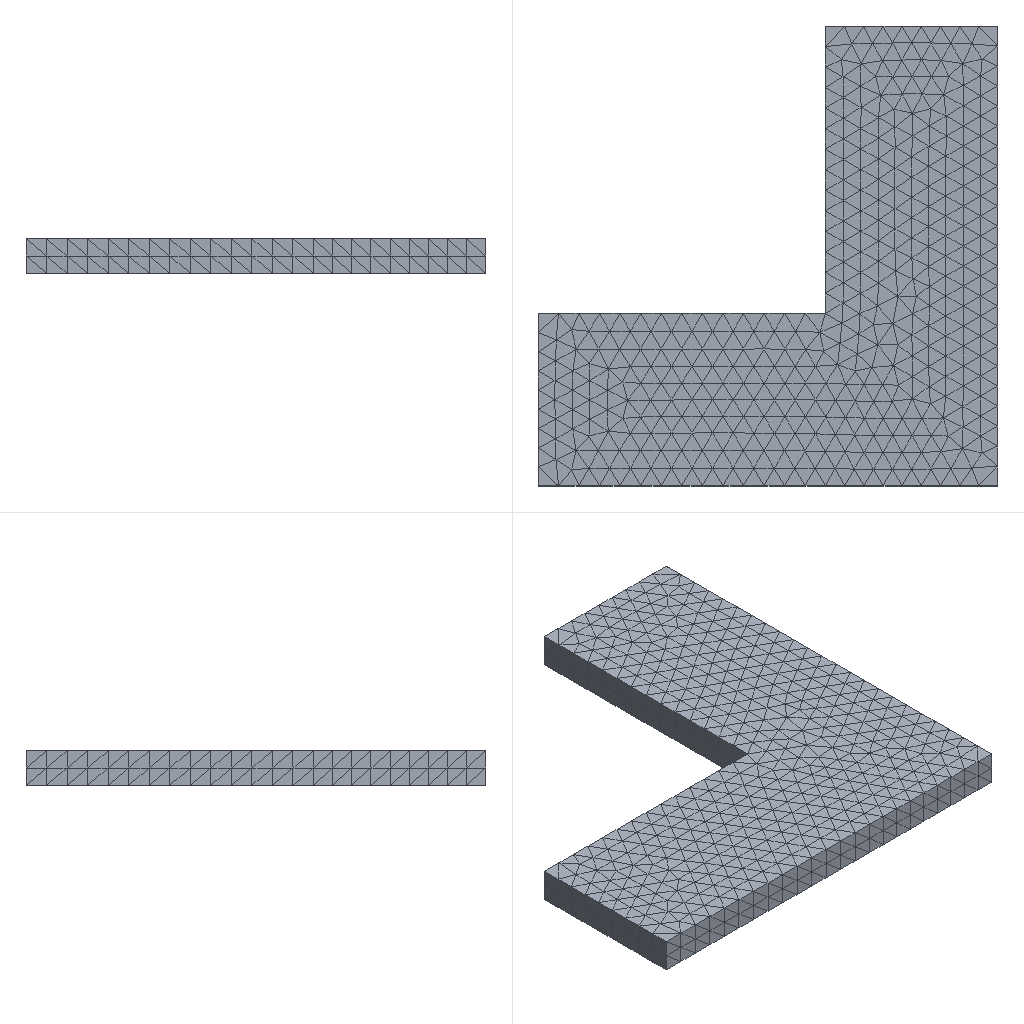Simulation study | abaqus
Notes in the study folder:
05 L bracket
job_status=None
Umax_mm=0.000139926
S_Mises_max_MPa=0.479355
Set-up summary:
category,name,step,type,value,unit,region
solver,abaqus,,Abaqus/CAE 2024
units,mm-N-s-tonne (MPa),,inferred,E=210000 density=7.85e-09
analysis,Step-1,,static,time_period=1
mesh,nodes,,,8082
mesh,elements,,,4612
element_type,C3D10,,,4612
material,Steel,,E,210000
material,Steel,,nu,0.3
material,Steel,,density,7.85e-09
section,Steel,,solid section,,,_PickedSet2
load,Load,Step-1,pressure,0.3,,LOAD
bc,BC,Step-1,encastre,[dofs=ENCASTRE],,FIXED
Abaqus input file, long lists of numbers shortened:
*Heading
** Job name: deck Model name: M05
** Generated by: Abaqus/CAE 2024
*Preprint, echo=NO, model=NO, history=NO, contact=NO
**
** PARTS
**
*Part, name=P
*Node
      1,         -50.,          30.,           6.
      2,           0.,          30.,           6.
** (8080 more lines like these left out)
*Element, type=C3D10
   1,  924,  925,  926,  802, 1278, 1277, 1276, 1280, 1279, 1281
   2,  802,  924,  859,  886, 1280, 1283, 1282, 1285, 1284, 1286
** (4610 more lines like these left out)
*Nset, nset=_PickedSet2, internal, generate
    1,  8082,     1
*Elset, elset=_PickedSet2, internal, generate
    1,  4612,     1
** Section: Sec
*Solid Section, elset=_PickedSet2, material=Steel
,
*End Part
**
**
** ASSEMBLY
**
*Assembly, name=Assembly
**
*Instance, name=I, part=P
*End Instance
**
*Nset, nset=FIXED, instance=I
    9,   10,   12,   14,   95,  117,  118,  119,  120,  121,  122,  123,  124,  125,  126,  127
  128,  129,  130,  131,  132,  133,  134,  135,  136,  137,  138,  147,  169,  170,  171,  172
** (13 more lines like these left out)
*Elset, elset=FIXED, instance=I
    9,   15,  105,  193,  194,  214,  244,  246,  330,  333,  335,  343,  364,  369,  396,  397
  419,  457,  459,  546,  635,  724,  959, 1077, 1078, 1129, 1141, 1153, 1156, 1207, 1211, 1299
** (4 more lines like these left out)
*Elset, elset=_LOAD_S3, internal, instance=I
  270,  374,  385,  387,  415,  924, 1457, 1458, 1736, 1808, 1814, 2365, 2383, 2389, 2390, 2395
 2397, 2411, 2417, 2422, 2423, 2438, 2451, 2454, 2461, 2470, 2479, 2735, 2746, 2748, 2755, 2901
** (1 more lines like these left out)
*Elset, elset=_LOAD_S1, internal, instance=I
 2372,
*Elset, elset=_LOAD_S4, internal, instance=I
 2915,
*Surface, type=ELEMENT, name=LOAD
_LOAD_S3, S3
_LOAD_S1, S1
_LOAD_S4, S4
*End Assembly
**
** MATERIALS
**
*Material, name=Steel
*Density
 7.85e-09,
*Elastic
210000., 0.3
** ----------------------------------------------------------------
**
** STEP: Step-1
**
*Step, name=Step-1, nlgeom=NO
*Static
1., 1., 1e-05, 1.
**
** BOUNDARY CONDITIONS
**
** Name: BC Type: Symmetry/Antisymmetry/Encastre
*Boundary
FIXED, ENCASTRE
**
** LOADS
**
** Name: Load   Type: Pressure
*Dsload
LOAD, P, 0.3
**
** OUTPUT REQUESTS
**
*Restart, write, frequency=0
**
** FIELD OUTPUT: F-Output-1
**
*Output, field, variable=PRESELECT
**
** HISTORY OUTPUT: H-Output-1
**
*Output, history, variable=PRESELECT
*End Step
Results summary:
result,odb.job_status,,,JOB_STATUS_COMPLETED_SUCCESSFULLY,"consistent, unstated (Abaqus has no unit system)"
result,steps[0].procedure,Step-1,,*STATIC,"consistent, unstated (Abaqus has no unit system)"
result,steps[0].time_period,Step-1,,1,"consistent, unstated (Abaqus has no unit system)"
result,steps[0].n_frames,Step-1,,2,"consistent, unstated (Abaqus has no unit system)"
result,steps[0].last_frame.id,Step-1,,1,"consistent, unstated (Abaqus has no unit system)"
result,steps[0].last_frame.value,Step-1,,1,"consistent, unstated (Abaqus has no unit system)"
result,steps[0].last_frame.description,Step-1,,Increment      1: Step Time =    1.000,"consistent, unstated (Abaqus has no unit system)"
result,steps[0].completed,Step-1,,True,"consistent, unstated (Abaqus has no unit system)"
result,steps[0].max_U_magnitude,Step-1,,0.0001399,"consistent, unstated (Abaqus has no unit system)"
result,steps[0].max_S_mises,Step-1,,0.4794,"consistent, unstated (Abaqus has no unit system)"
result,steps[0].RF_sum[1],Step-1,,-54,"consistent, unstated (Abaqus has no unit system)"
result,steps[0].RF_sum[2],Step-1,,1.44355e-07,"consistent, unstated (Abaqus has no unit system)"
result,steps[0].RF_sum[3],Step-1,,-1.15251e-07,"consistent, unstated (Abaqus has no unit system)"
result,steps[1].procedure,Step-1,,*STATIC,"consistent, unstated (Abaqus has no unit system)"
result,steps[1].time_period,Step-1,,1,"consistent, unstated (Abaqus has no unit system)"
result,steps[1].n_frames,Step-1,,2,"consistent, unstated (Abaqus has no unit system)"
result,steps[1].last_frame.id,Step-1,,1,"consistent, unstated (Abaqus has no unit system)"
result,steps[1].last_frame.value,Step-1,,1,"consistent, unstated (Abaqus has no unit system)"
result,steps[1].last_frame.description,Step-1,,Increment      1: Step Time =    1.000,"consistent, unstated (Abaqus has no unit system)"
result,steps[1].completed,Step-1,,True,"consistent, unstated (Abaqus has no unit system)"
result,steps[1].max_U_magnitude,Step-1,,0.0001399,"consistent, unstated (Abaqus has no unit system)"
result,steps[1].max_S_mises,Step-1,,0.4794,"consistent, unstated (Abaqus has no unit system)"
result,steps[1].RF_sum[1],Step-1,,-54,"consistent, unstated (Abaqus has no unit system)"
result,steps[1].RF_sum[2],Step-1,,1.44355e-07,"consistent, unstated (Abaqus has no unit system)"
result,steps[1].RF_sum[3],Step-1,,-1.15251e-07,"consistent, unstated (Abaqus has no unit system)"